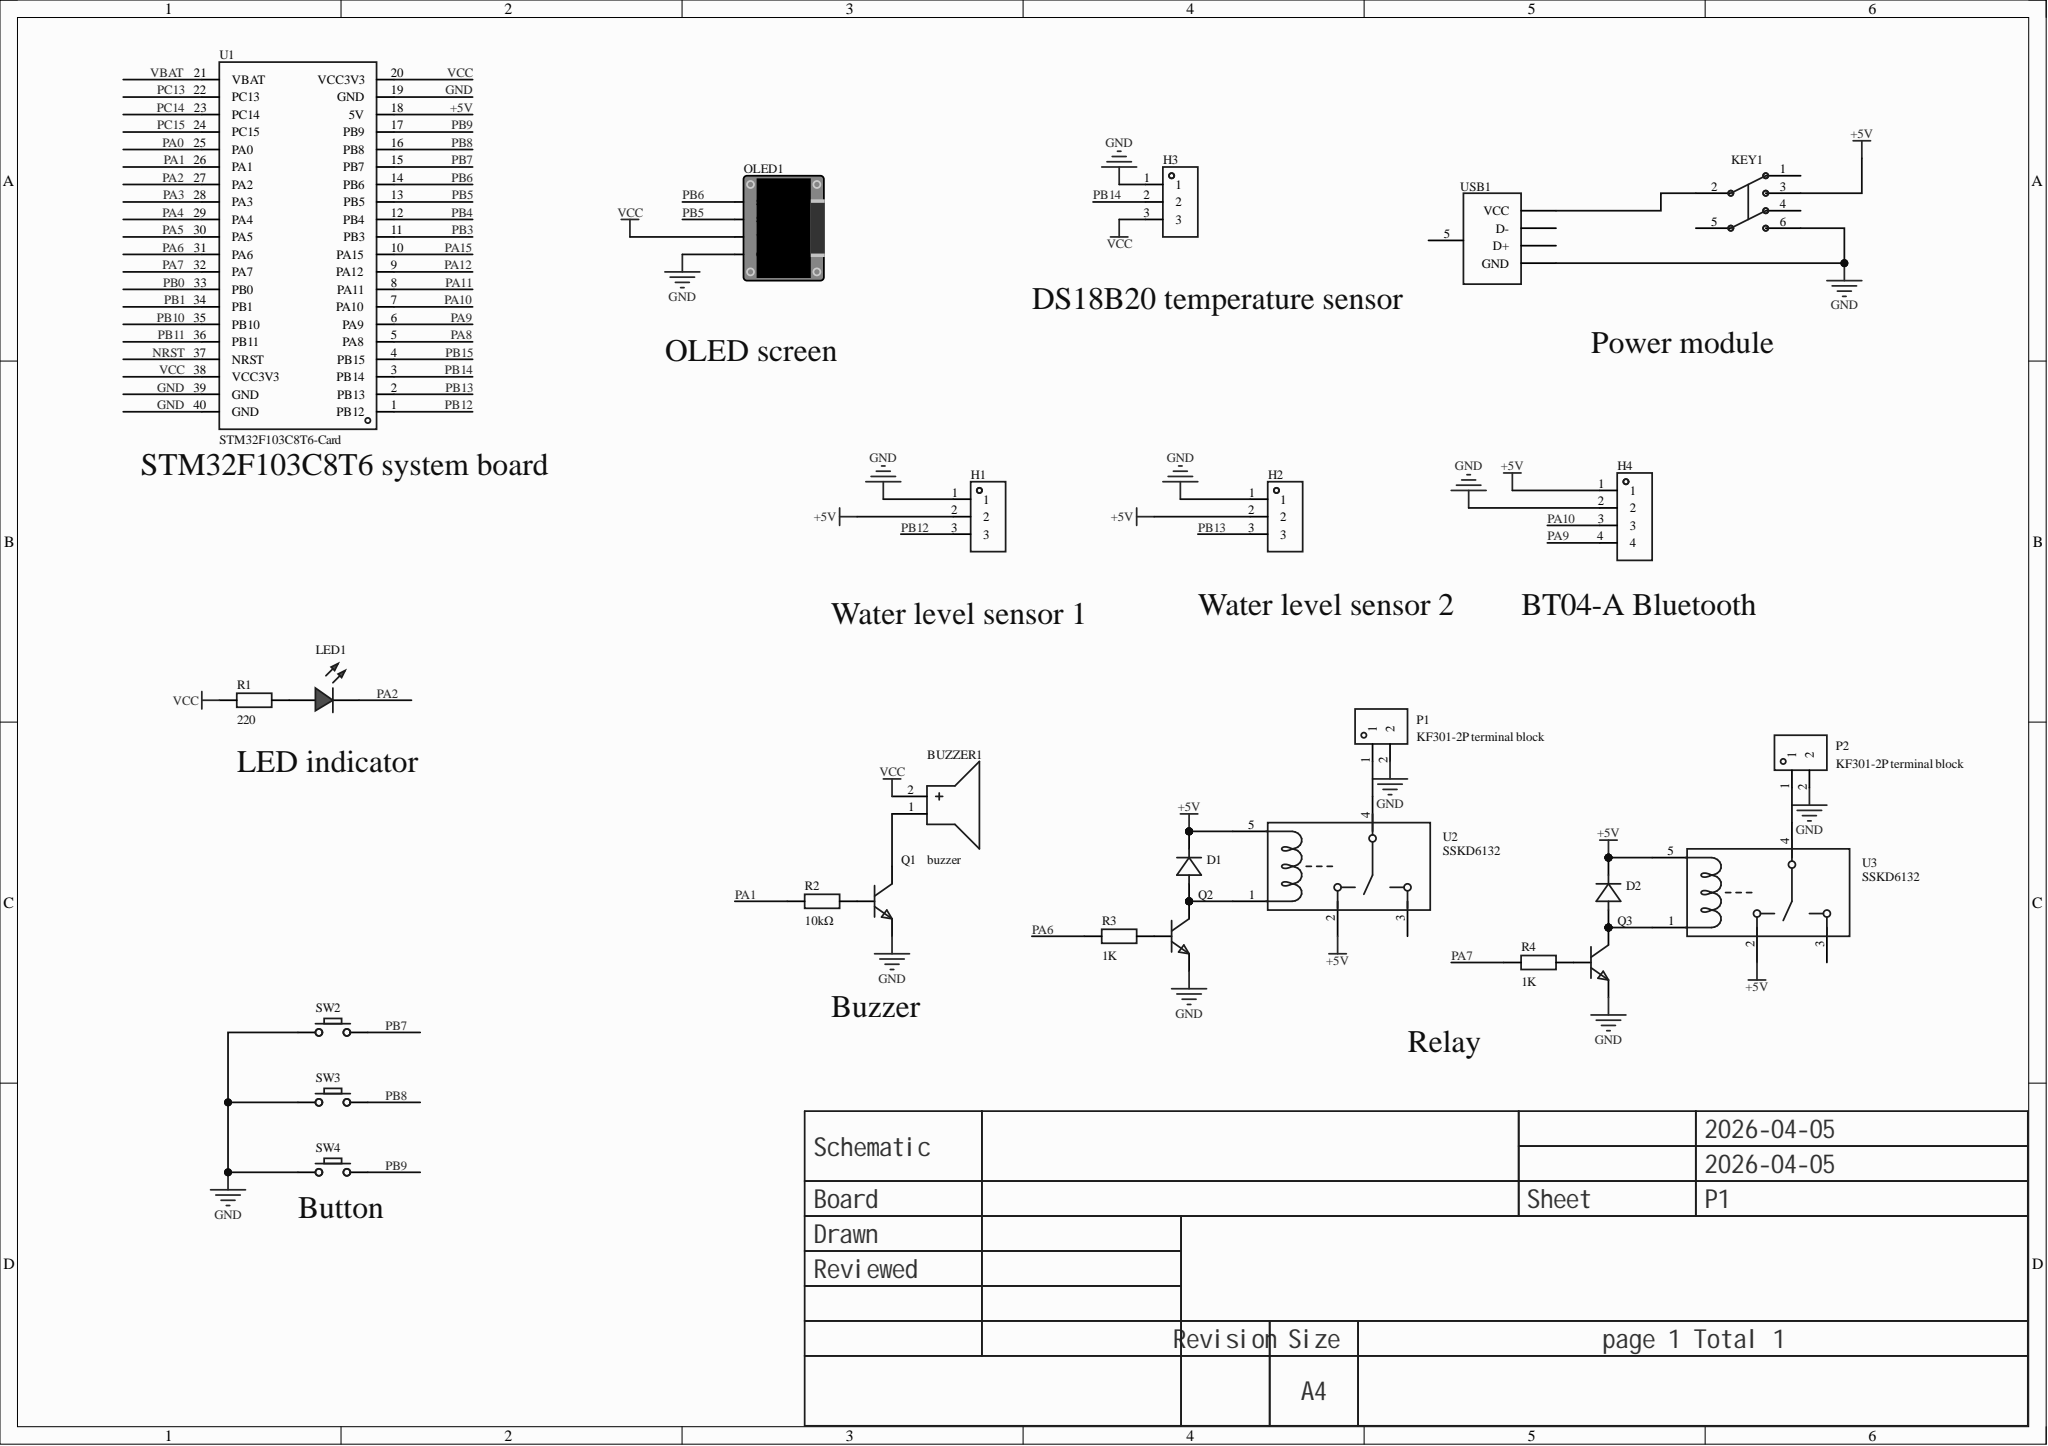Circuit board | Altium Designer | 26 parts | 27 nets
Bill of materials:
Comment,Description,Designator,Footprint,LibRef,Quantity
"buzzer","","BUZZER1","BUZ-TH_BD12.0-P6.00-D0.9-RD","buzzer","1"
"","","D1, D2","SMA_1N4007","D_1N4007","2"
"","","H1, H2, H3","HDR-TH_3P-P2.54-V-F","HDR-F_2.54_1x3P","3"
"","","H4","HDR-TH_4P-P2.54-V-F","HDR-F_2.54_1x4P","1"
"Non-self-locking switch 8.5×8.5 silent","6-pin, 8.5×8.5","KEY1","SW-TH_6P-L8.5-W8.5-P2.54","无自锁开关 8.5×8.5 无声","1"
"","","LED1","LED_TH-3mm","LED_TH-R_3mm","1"
"","","OLED1","0.96OLED_4P","0.96OLED模块_4P","1"
"KF301-2P terminal block","","P1, P2","CONN-TH_XY301V-A-5.0-2P","KF301-2P接线端子","2"
"","","Q1","S8050_TO_92","S8050_TO_NPN","1"
"","","Q2, Q3","S8050_SOT-23","S8050_SOT_NPN","2"
"220","","R1","Res_1/8W","Res_AXIAL-1/8W","1"
"10kΩ","","R2","Res_1/8W","Res_AXIAL-1/8W","1"
"1K","","R3, R4","R0603","Res_0603","2"
"","","SW2, SW3, SW4","Key_TH_3.5x6x4.3","Key_TH_3.5x6x4.3","3"
"STM32F103C8T6-Card","","U1","CONN-TH_L53.3-W22.9_STM32F103C8T6-CARD","STM32F103C8T6-Card","1"
"SSKD6132","","U2, U3","RELAY-TH_G2R-1","SSKD6132","2"
"","","USB1","USB_ Type-B","USB_ Type-B","1"
Netlist (Protel format):
[
BUZZER1
BUZ-TH_BD12.0-P6.00-D0.9-RD
buzzer



]
[
D1
SMA_1N4007




]
[
D2
SMA_1N4007




]
[
H1
HDR-TH_3P-P2.54-V-F




]
[
H2
HDR-TH_3P-P2.54-V-F




]
[
H3
HDR-TH_3P-P2.54-V-F




]
[
H4
HDR-TH_4P-P2.54-V-F




]
[
KEY1
SW-TH_6P-L8.5-W8.5-P2.54
Non-self-locking switch 8.5×8.5 silent



]
[
LED1
LED_TH-3mm




]
[
OLED1
0.96OLED_4P




]
[
P1
CONN-TH_XY301V-A-5.0-2P
KF301-2P terminal block



]
[
P2
CONN-TH_XY301V-A-5.0-2P
KF301-2P terminal block



]
[
Q1
S8050_TO_92




]
[
Q2
S8050_SOT-23




]
[
Q3
S8050_SOT-23




]
[
R1
Res_1/8W
220



]
[
R2
Res_1/8W
10kΩ



]
[
R3
R0603
1K



]
[
R4
R0603
1K



]
[
SW2
Key_TH_3.5x6x4.3




]
[
SW3
Key_TH_3.5x6x4.3




]
[
SW4
Key_TH_3.5x6x4.3




]
[
U1
CONN-TH_L53.3-W22.9_STM32F103C8T6-CARD
STM32F103C8T6-Card



]
[
U2
RELAY-TH_G2R-1
SSKD6132



]
[
U3
RELAY-TH_G2R-1
SSKD6132



]
[
USB1
USB_ Type-B




]
(
VCC
BUZZER1-2
H3-3
OLED1-2
R1-1
U1-20
U1-38
)
(
PB14
H3-2
U1-3
)
(
PB13
H2-3
U1-2
)
(
PB12
H1-3
U1-1
)
(
PB9
SW4-B
U1-17
)
(
PB8
SW3-B
U1-16
)
(
PB7
SW2-B
U1-15
)
(
PB6
OLED1-4
U1-14
)
(
PB5
OLED1-3
U1-13
)
(
PA10
H4-3
U1-7
)
(
PA9
H4-4
U1-6
)
(
PA7
R4-1
U1-32
)
(
PA6
R3-1
U1-31
)
(
PA2
LED1-2
U1-27
)
(
PA1
R2-1
U1-26
)
(
NetQ3_1
Q3-1
R4-2
)
(
NetQ2_1
Q2-1
R3-2
)
(
NetQ1_2
Q1-2
R2-2
)
(
NetP2_1
P2-1
U3-4
)
(
NetP1_1
P1-1
U2-4
)
(
NetLED1_1
LED1-1
R1-2
)
(
NetKEY1_2
KEY1-2
USB1-1
)
(
NetD2_2
D2-2
Q3-3
U3-1
)
(
NetD1_2
D1-2
Q2-3
U2-1
)
(
NetBUZZER1_1
BUZZER1-1
Q1-3
)
(
GND
H1-1
H2-1
H3-1
H4-2
KEY1-6
OLED1-1
P1-2
P2-2
Q1-1
Q2-2
Q3-2
SW2-A
SW3-A
SW4-A
U1-19
U1-39
U1-40
USB1-4
)
(
+5V
D1-1
D2-1
H1-2
H2-2
H4-1
KEY1-3
U1-18
U2-2
U2-5
U3-2
U3-5
)